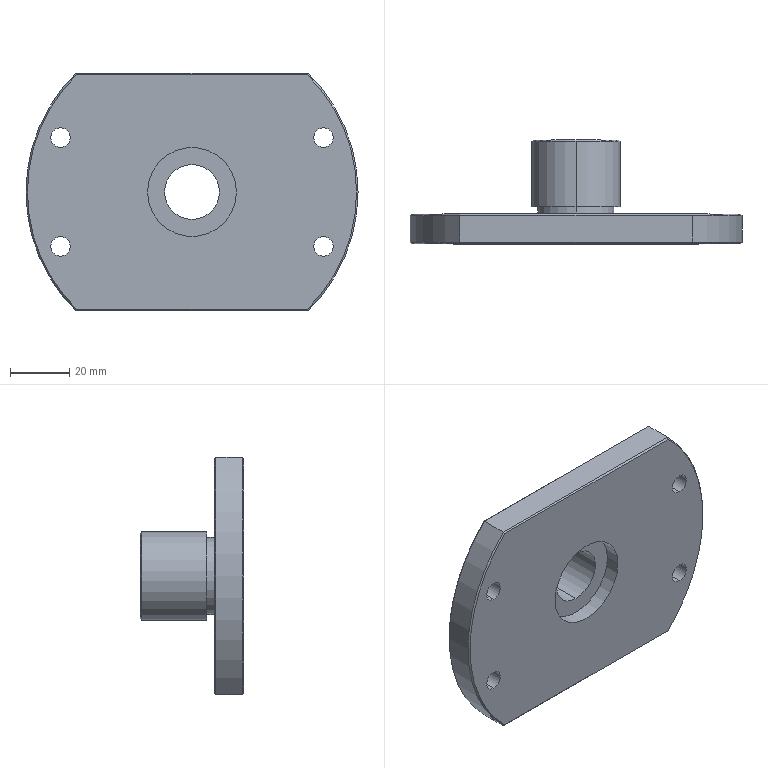Part | SolidWorks | features ICE 3, HoleWzd 2, Chamfer 1, Extrusion 1, RevCut 1 | 1 solid | 43 faces | box 112 x 35 x 80 mm | volume 84771 mm3 | cylinder 18 | cone 14 | plane 11 | commonest cylinder face diameters 6.6 x8 30 x4 18.5 x2 26 x2 112 x2
STEP:
#1=CARTESIAN_POINT('',(-15.,5.,0.));
#2=VERTEX_POINT('',#1);
#3=CARTESIAN_POINT('',(15.,5.,0.));
#4=VERTEX_POINT('',#3);
#5=CARTESIAN_POINT('',(0.,5.,0.));
#6=DIRECTION('',(0.,-1.,0.));
#7=DIRECTION('',(1.,0.,0.));
#8=AXIS2_PLACEMENT_3D('',#5,#6,#7);
#9=CIRCLE('',#8,15.);
#10=EDGE_CURVE('',#2,#4,#9,.T.);
#11=ORIENTED_EDGE('',*,*,#10,.F.);
#12=CARTESIAN_POINT('',(-15.,0.,0.));
#13=VERTEX_POINT('',#12);
#14=CARTESIAN_POINT('',(-15.,5.,0.));
#15=DIRECTION('',(0.,-1.,0.));
#16=VECTOR('',#15,1000.);
#17=LINE('',#14,#16);
#18=EDGE_CURVE('',#2,#13,#17,.T.);
#19=ORIENTED_EDGE('',*,*,#18,.T.);
#20=CARTESIAN_POINT('',(15.,0.,0.));
#21=VERTEX_POINT('',#20);
#22=CARTESIAN_POINT('',(0.,0.,0.));
#23=DIRECTION('',(0.,-1.,0.));
#24=DIRECTION('',(1.,0.,0.));
#25=AXIS2_PLACEMENT_3D('',#22,#23,#24);
#26=CIRCLE('',#25,15.);
#27=EDGE_CURVE('',#13,#21,#26,.T.);
#28=ORIENTED_EDGE('',*,*,#27,.T.);
#29=CARTESIAN_POINT('',(15.,5.,0.));
#30=DIRECTION('',(0.,-1.,0.));
#31=VECTOR('',#30,1000.);
#32=LINE('',#29,#31);
#33=EDGE_CURVE('',#4,#21,#32,.T.);
#34=ORIENTED_EDGE('',*,*,#33,.F.);
#35=EDGE_LOOP('',(#11,#19,#28,#34));
#36=FACE_OUTER_BOUND('',#35,.T.);
#37=CARTESIAN_POINT('',(0.,5.,0.));
#38=DIRECTION('',(0.,-1.,0.));
#39=DIRECTION('',(1.,0.,0.));
#40=AXIS2_PLACEMENT_3D('',#37,#38,#39);
#41=CYLINDRICAL_SURFACE('',#40,15.);
#42=ADVANCED_FACE('',(#36),#41,.F.);
#43=CARTESIAN_POINT('',(0.,35.,14.5));
#44=VERTEX_POINT('',#43);
#45=CARTESIAN_POINT('',(0.,35.,-14.5));
#46=VERTEX_POINT('',#45);
#47=CARTESIAN_POINT('',(0.,35.,0.));
#48=DIRECTION('',(0.,1.,0.));
#49=DIRECTION('',(0.,0.,1.));
#50=AXIS2_PLACEMENT_3D('',#47,#48,#49);
#51=CIRCLE('',#50,14.5);
#52=EDGE_CURVE('',#44,#46,#51,.T.);
#53=ORIENTED_EDGE('',*,*,#52,.F.);
#54=CARTESIAN_POINT('',(0.,34.5,15.));
#55=VERTEX_POINT('',#54);
#56=CARTESIAN_POINT('',(0.,35.,14.5));
#57=DIRECTION('',(0.,-0.7071,0.7071));
#58=VECTOR('',#57,1000.);
#59=LINE('',#56,#58);
#60=EDGE_CURVE('',#44,#55,#59,.T.);
#61=ORIENTED_EDGE('',*,*,#60,.T.);
#62=CARTESIAN_POINT('',(0.,34.5,-15.));
#63=VERTEX_POINT('',#62);
#64=CARTESIAN_POINT('',(0.,34.5,0.));
#65=DIRECTION('',(0.,-1.,0.));
#66=DIRECTION('',(0.,0.,1.));
#67=AXIS2_PLACEMENT_3D('',#64,#65,#66);
#68=CIRCLE('',#67,15.);
#69=EDGE_CURVE('',#63,#55,#68,.T.);
#70=ORIENTED_EDGE('',*,*,#69,.F.);
#71=CARTESIAN_POINT('',(0.,35.,-14.5));
#72=DIRECTION('',(0.,-0.7071,-0.7071));
#73=VECTOR('',#72,1000.);
#74=LINE('',#71,#73);
#75=EDGE_CURVE('',#46,#63,#74,.T.);
#76=ORIENTED_EDGE('',*,*,#75,.F.);
#77=EDGE_LOOP('',(#53,#61,#70,#76));
#78=FACE_OUTER_BOUND('',#77,.T.);
#79=CARTESIAN_POINT('',(0.,35.,0.));
#80=DIRECTION('',(0.,-1.,0.));
#81=DIRECTION('',(0.,0.,-1.));
#82=AXIS2_PLACEMENT_3D('',#79,#80,#81);
#83=CONICAL_SURFACE('',#82,14.5,0.7854);
#84=ADVANCED_FACE('',(#78),#83,.T.);
#85=CARTESIAN_POINT('',(0.,12.5,-13.));
#86=VERTEX_POINT('',#85);
#87=CARTESIAN_POINT('',(0.,12.5,13.));
#88=VERTEX_POINT('',#87);
#89=CARTESIAN_POINT('',(0.,12.5,0.));
#90=DIRECTION('',(0.,-1.,0.));
#91=DIRECTION('',(0.,0.,-1.));
#92=AXIS2_PLACEMENT_3D('',#89,#90,#91);
#93=CIRCLE('',#92,13.);
#94=EDGE_CURVE('',#86,#88,#93,.T.);
#95=ORIENTED_EDGE('',*,*,#94,.T.);
#96=CARTESIAN_POINT('',(0.,10.,13.));
#97=VERTEX_POINT('',#96);
#98=CARTESIAN_POINT('',(0.,-2.797,13.));
#99=DIRECTION('',(0.,-1.,0.));
#100=VECTOR('',#99,1000.);
#101=LINE('',#98,#100);
#102=EDGE_CURVE('',#88,#97,#101,.T.);
#103=ORIENTED_EDGE('',*,*,#102,.T.);
#104=CARTESIAN_POINT('',(0.,10.,-13.));
#105=VERTEX_POINT('',#104);
#106=CARTESIAN_POINT('',(0.,10.,0.));
#107=DIRECTION('',(0.,-1.,0.));
#108=DIRECTION('',(0.,0.,-1.));
#109=AXIS2_PLACEMENT_3D('',#106,#107,#108);
#110=CIRCLE('',#109,13.);
#111=EDGE_CURVE('',#105,#97,#110,.T.);
#112=ORIENTED_EDGE('',*,*,#111,.F.);
#113=CARTESIAN_POINT('',(0.,-2.797,-13.));
#114=DIRECTION('',(0.,-1.,0.));
#115=VECTOR('',#114,1000.);
#116=LINE('',#113,#115);
#117=EDGE_CURVE('',#86,#105,#116,.T.);
#118=ORIENTED_EDGE('',*,*,#117,.F.);
#119=EDGE_LOOP('',(#95,#103,#112,#118));
#120=FACE_OUTER_BOUND('',#119,.T.);
#121=CARTESIAN_POINT('',(0.,-2.797,0.));
#122=DIRECTION('',(0.,-1.,0.));
#123=DIRECTION('',(0.,0.,-1.));
#124=AXIS2_PLACEMENT_3D('',#121,#122,#123);
#125=CYLINDRICAL_SURFACE('',#124,13.);
#126=ADVANCED_FACE('',(#120),#125,.T.);
#127=CARTESIAN_POINT('',(44.346,6.58,15.069));
#128=VERTEX_POINT('',#127);
#129=CARTESIAN_POINT('',(44.346,6.58,21.669));
#130=VERTEX_POINT('',#129);
#131=CARTESIAN_POINT('',(44.346,6.58,18.369));
#132=DIRECTION('',(0.,1.,0.));
#133=DIRECTION('',(0.,0.,1.));
#134=AXIS2_PLACEMENT_3D('',#131,#132,#133);
#135=CIRCLE('',#134,3.3);
#136=EDGE_CURVE('',#128,#130,#135,.T.);
#137=ORIENTED_EDGE('',*,*,#136,.F.);
#138=CARTESIAN_POINT('',(44.346,10.,11.649));
#139=VERTEX_POINT('',#138);
#140=CARTESIAN_POINT('',(44.346,10.,11.649));
#141=DIRECTION('',(0.,0.7071,-0.7071));
#142=VECTOR('',#141,1000.);
#143=LINE('',#140,#142);
#144=EDGE_CURVE('',#128,#139,#143,.T.);
#145=ORIENTED_EDGE('',*,*,#144,.T.);
#146=CARTESIAN_POINT('',(44.346,10.,25.089));
#147=VERTEX_POINT('',#146);
#148=CARTESIAN_POINT('',(44.346,10.,18.369));
#149=DIRECTION('',(0.,1.,0.));
#150=DIRECTION('',(0.,0.,1.));
#151=AXIS2_PLACEMENT_3D('',#148,#149,#150);
#152=CIRCLE('',#151,6.72);
#153=EDGE_CURVE('',#139,#147,#152,.T.);
#154=ORIENTED_EDGE('',*,*,#153,.T.);
#155=CARTESIAN_POINT('',(44.346,10.,25.089));
#156=DIRECTION('',(0.,0.7071,0.7071));
#157=VECTOR('',#156,1000.);
#158=LINE('',#155,#157);
#159=EDGE_CURVE('',#130,#147,#158,.T.);
#160=ORIENTED_EDGE('',*,*,#159,.F.);
#161=EDGE_LOOP('',(#137,#145,#154,#160));
#162=FACE_OUTER_BOUND('',#161,.T.);
#163=CARTESIAN_POINT('',(44.346,10.,18.369));
#164=DIRECTION('',(0.,1.,0.));
#165=DIRECTION('',(0.,0.,1.));
#166=AXIS2_PLACEMENT_3D('',#163,#164,#165);
#167=CONICAL_SURFACE('',#166,6.72,0.7854);
#168=ADVANCED_FACE('',(#162),#167,.F.);
#169=CARTESIAN_POINT('',(44.346,0.,15.069));
#170=VERTEX_POINT('',#169);
#171=CARTESIAN_POINT('',(44.346,0.,21.669));
#172=VERTEX_POINT('',#171);
#173=CARTESIAN_POINT('',(44.346,0.,18.369));
#174=DIRECTION('',(0.,1.,0.));
#175=DIRECTION('',(0.,0.,1.));
#176=AXIS2_PLACEMENT_3D('',#173,#174,#175);
#177=CIRCLE('',#176,3.3);
#178=EDGE_CURVE('',#170,#172,#177,.T.);
#179=ORIENTED_EDGE('',*,*,#178,.F.);
#180=CARTESIAN_POINT('',(44.346,10.,15.069));
#181=DIRECTION('',(0.,1.,0.));
#182=VECTOR('',#181,1000.);
#183=LINE('',#180,#182);
#184=EDGE_CURVE('',#170,#128,#183,.T.);
#185=ORIENTED_EDGE('',*,*,#184,.T.);
#186=ORIENTED_EDGE('',*,*,#136,.T.);
#187=CARTESIAN_POINT('',(44.346,10.,21.669));
#188=DIRECTION('',(0.,1.,0.));
#189=VECTOR('',#188,1000.);
#190=LINE('',#187,#189);
#191=EDGE_CURVE('',#172,#130,#190,.T.);
#192=ORIENTED_EDGE('',*,*,#191,.F.);
#193=EDGE_LOOP('',(#179,#185,#186,#192));
#194=FACE_OUTER_BOUND('',#193,.T.);
#195=CARTESIAN_POINT('',(44.346,10.,18.369));
#196=DIRECTION('',(0.,1.,0.));
#197=DIRECTION('',(0.,0.,1.));
#198=AXIS2_PLACEMENT_3D('',#195,#196,#197);
#199=CYLINDRICAL_SURFACE('',#198,3.3);
#200=ADVANCED_FACE('',(#194),#199,.F.);
#201=CARTESIAN_POINT('',(-44.346,6.58,-21.669));
#202=VERTEX_POINT('',#201);
#203=CARTESIAN_POINT('',(-44.346,6.58,-15.069));
#204=VERTEX_POINT('',#203);
#205=CARTESIAN_POINT('',(-44.346,6.58,-18.369));
#206=DIRECTION('',(0.,1.,0.));
#207=DIRECTION('',(0.,0.,1.));
#208=AXIS2_PLACEMENT_3D('',#205,#206,#207);
#209=CIRCLE('',#208,3.3);
#210=EDGE_CURVE('',#202,#204,#209,.T.);
#211=ORIENTED_EDGE('',*,*,#210,.F.);
#212=CARTESIAN_POINT('',(-44.346,10.,-25.089));
#213=VERTEX_POINT('',#212);
#214=CARTESIAN_POINT('',(-44.346,10.,-25.089));
#215=DIRECTION('',(0.,0.7071,-0.7071));
#216=VECTOR('',#215,1000.);
#217=LINE('',#214,#216);
#218=EDGE_CURVE('',#202,#213,#217,.T.);
#219=ORIENTED_EDGE('',*,*,#218,.T.);
#220=CARTESIAN_POINT('',(-44.346,10.,-11.649));
#221=VERTEX_POINT('',#220);
#222=CARTESIAN_POINT('',(-44.346,10.,-18.369));
#223=DIRECTION('',(0.,1.,0.));
#224=DIRECTION('',(0.,0.,1.));
#225=AXIS2_PLACEMENT_3D('',#222,#223,#224);
#226=CIRCLE('',#225,6.72);
#227=EDGE_CURVE('',#213,#221,#226,.T.);
#228=ORIENTED_EDGE('',*,*,#227,.T.);
#229=CARTESIAN_POINT('',(-44.346,10.,-11.649));
#230=DIRECTION('',(0.,0.7071,0.7071));
#231=VECTOR('',#230,1000.);
#232=LINE('',#229,#231);
#233=EDGE_CURVE('',#204,#221,#232,.T.);
#234=ORIENTED_EDGE('',*,*,#233,.F.);
#235=EDGE_LOOP('',(#211,#219,#228,#234));
#236=FACE_OUTER_BOUND('',#235,.T.);
#237=CARTESIAN_POINT('',(-44.346,10.,-18.369));
#238=DIRECTION('',(0.,1.,0.));
#239=DIRECTION('',(0.,0.,1.));
#240=AXIS2_PLACEMENT_3D('',#237,#238,#239);
#241=CONICAL_SURFACE('',#240,6.72,0.7854);
#242=ADVANCED_FACE('',(#236),#241,.F.);
#243=CARTESIAN_POINT('',(-44.346,0.,-21.669));
#244=VERTEX_POINT('',#243);
#245=CARTESIAN_POINT('',(-44.346,0.,-15.069));
#246=VERTEX_POINT('',#245);
#247=CARTESIAN_POINT('',(-44.346,0.,-18.369));
#248=DIRECTION('',(0.,1.,0.));
#249=DIRECTION('',(0.,0.,1.));
#250=AXIS2_PLACEMENT_3D('',#247,#248,#249);
#251=CIRCLE('',#250,3.3);
#252=EDGE_CURVE('',#244,#246,#251,.T.);
#253=ORIENTED_EDGE('',*,*,#252,.F.);
#254=CARTESIAN_POINT('',(-44.346,10.,-21.669));
#255=DIRECTION('',(0.,1.,0.));
#256=VECTOR('',#255,1000.);
#257=LINE('',#254,#256);
#258=EDGE_CURVE('',#244,#202,#257,.T.);
#259=ORIENTED_EDGE('',*,*,#258,.T.);
#260=ORIENTED_EDGE('',*,*,#210,.T.);
#261=CARTESIAN_POINT('',(-44.346,10.,-15.069));
#262=DIRECTION('',(0.,1.,0.));
#263=VECTOR('',#262,1000.);
#264=LINE('',#261,#263);
#265=EDGE_CURVE('',#246,#204,#264,.T.);
#266=ORIENTED_EDGE('',*,*,#265,.F.);
#267=EDGE_LOOP('',(#253,#259,#260,#266));
#268=FACE_OUTER_BOUND('',#267,.T.);
#269=CARTESIAN_POINT('',(-44.346,10.,-18.369));
#270=DIRECTION('',(0.,1.,0.));
#271=DIRECTION('',(0.,0.,1.));
#272=AXIS2_PLACEMENT_3D('',#269,#270,#271);
#273=CYLINDRICAL_SURFACE('',#272,3.3);
#274=ADVANCED_FACE('',(#268),#273,.F.);
#275=CARTESIAN_POINT('',(-44.346,6.58,15.069));
#276=VERTEX_POINT('',#275);
#277=CARTESIAN_POINT('',(-44.346,6.58,21.669));
#278=VERTEX_POINT('',#277);
#279=CARTESIAN_POINT('',(-44.346,6.58,18.369));
#280=DIRECTION('',(0.,1.,0.));
#281=DIRECTION('',(0.,0.,1.));
#282=AXIS2_PLACEMENT_3D('',#279,#280,#281);
#283=CIRCLE('',#282,3.3);
#284=EDGE_CURVE('',#276,#278,#283,.T.);
#285=ORIENTED_EDGE('',*,*,#284,.F.);
#286=CARTESIAN_POINT('',(-44.346,10.,11.649));
#287=VERTEX_POINT('',#286);
#288=CARTESIAN_POINT('',(-44.346,10.,11.649));
#289=DIRECTION('',(0.,0.7071,-0.7071));
#290=VECTOR('',#289,1000.);
#291=LINE('',#288,#290);
#292=EDGE_CURVE('',#276,#287,#291,.T.);
#293=ORIENTED_EDGE('',*,*,#292,.T.);
#294=CARTESIAN_POINT('',(-44.346,10.,25.089));
#295=VERTEX_POINT('',#294);
#296=CARTESIAN_POINT('',(-44.346,10.,18.369));
#297=DIRECTION('',(0.,1.,0.));
#298=DIRECTION('',(0.,0.,1.));
#299=AXIS2_PLACEMENT_3D('',#296,#297,#298);
#300=CIRCLE('',#299,6.72);
#301=EDGE_CURVE('',#287,#295,#300,.T.);
#302=ORIENTED_EDGE('',*,*,#301,.T.);
#303=CARTESIAN_POINT('',(-44.346,10.,25.089));
#304=DIRECTION('',(0.,0.7071,0.7071));
#305=VECTOR('',#304,1000.);
#306=LINE('',#303,#305);
#307=EDGE_CURVE('',#278,#295,#306,.T.);
#308=ORIENTED_EDGE('',*,*,#307,.F.);
#309=EDGE_LOOP('',(#285,#293,#302,#308));
#310=FACE_OUTER_BOUND('',#309,.T.);
#311=CARTESIAN_POINT('',(-44.346,10.,18.369));
#312=DIRECTION('',(0.,1.,0.));
#313=DIRECTION('',(0.,0.,1.));
#314=AXIS2_PLACEMENT_3D('',#311,#312,#313);
#315=CONICAL_SURFACE('',#314,6.72,0.7854);
#316=ADVANCED_FACE('',(#310),#315,.F.);
#317=CARTESIAN_POINT('',(-44.346,0.,15.069));
#318=VERTEX_POINT('',#317);
#319=CARTESIAN_POINT('',(-44.346,0.,21.669));
#320=VERTEX_POINT('',#319);
#321=CARTESIAN_POINT('',(-44.346,0.,18.369));
#322=DIRECTION('',(0.,1.,0.));
#323=DIRECTION('',(0.,0.,1.));
#324=AXIS2_PLACEMENT_3D('',#321,#322,#323);
#325=CIRCLE('',#324,3.3);
#326=EDGE_CURVE('',#318,#320,#325,.T.);
#327=ORIENTED_EDGE('',*,*,#326,.F.);
#328=CARTESIAN_POINT('',(-44.346,10.,15.069));
#329=DIRECTION('',(0.,1.,0.));
#330=VECTOR('',#329,1000.);
#331=LINE('',#328,#330);
#332=EDGE_CURVE('',#318,#276,#331,.T.);
#333=ORIENTED_EDGE('',*,*,#332,.T.);
#334=ORIENTED_EDGE('',*,*,#284,.T.);
#335=CARTESIAN_POINT('',(-44.346,10.,21.669));
#336=DIRECTION('',(0.,1.,0.));
#337=VECTOR('',#336,1000.);
#338=LINE('',#335,#337);
#339=EDGE_CURVE('',#320,#278,#338,.T.);
#340=ORIENTED_EDGE('',*,*,#339,.F.);
#341=EDGE_LOOP('',(#327,#333,#334,#340));
#342=FACE_OUTER_BOUND('',#341,.T.);
#343=CARTESIAN_POINT('',(-44.346,10.,18.369));
#344=DIRECTION('',(0.,1.,0.));
#345=DIRECTION('',(0.,0.,1.));
#346=AXIS2_PLACEMENT_3D('',#343,#344,#345);
#347=CYLINDRICAL_SURFACE('',#346,3.3);
#348=ADVANCED_FACE('',(#342),#347,.F.);
#349=CARTESIAN_POINT('',(44.346,6.58,-21.669));
#350=VERTEX_POINT('',#349);
#351=CARTESIAN_POINT('',(44.346,6.58,-15.069));
#352=VERTEX_POINT('',#351);
#353=CARTESIAN_POINT('',(44.346,6.58,-18.369));
#354=DIRECTION('',(0.,1.,0.));
#355=DIRECTION('',(0.,0.,1.));
#356=AXIS2_PLACEMENT_3D('',#353,#354,#355);
#357=CIRCLE('',#356,3.3);
#358=EDGE_CURVE('',#350,#352,#357,.T.);
#359=ORIENTED_EDGE('',*,*,#358,.F.);
#360=CARTESIAN_POINT('',(44.346,10.,-25.089));
#361=VERTEX_POINT('',#360);
#362=CARTESIAN_POINT('',(44.346,10.,-25.089));
#363=DIRECTION('',(0.,0.7071,-0.7071));
#364=VECTOR('',#363,1000.);
#365=LINE('',#362,#364);
#366=EDGE_CURVE('',#350,#361,#365,.T.);
#367=ORIENTED_EDGE('',*,*,#366,.T.);
#368=CARTESIAN_POINT('',(44.346,10.,-11.649));
#369=VERTEX_POINT('',#368);
#370=CARTESIAN_POINT('',(44.346,10.,-18.369));
#371=DIRECTION('',(0.,1.,0.));
#372=DIRECTION('',(0.,0.,1.));
#373=AXIS2_PLACEMENT_3D('',#370,#371,#372);
#374=CIRCLE('',#373,6.72);
#375=EDGE_CURVE('',#361,#369,#374,.T.);
#376=ORIENTED_EDGE('',*,*,#375,.T.);
#377=CARTESIAN_POINT('',(44.346,10.,-11.649));
#378=DIRECTION('',(0.,0.7071,0.7071));
#379=VECTOR('',#378,1000.);
#380=LINE('',#377,#379);
#381=EDGE_CURVE('',#352,#369,#380,.T.);
#382=ORIENTED_EDGE('',*,*,#381,.F.);
#383=EDGE_LOOP('',(#359,#367,#376,#382));
#384=FACE_OUTER_BOUND('',#383,.T.);
#385=CARTESIAN_POINT('',(44.346,10.,-18.369));
#386=DIRECTION('',(0.,1.,0.));
#387=DIRECTION('',(0.,0.,1.));
#388=AXIS2_PLACEMENT_3D('',#385,#386,#387);
#389=CONICAL_SURFACE('',#388,6.72,0.7854);
#390=ADVANCED_FACE('',(#384),#389,.F.);
#391=CARTESIAN_POINT('',(44.346,0.,-21.669));
#392=VERTEX_POINT('',#391);
#393=CARTESIAN_POINT('',(44.346,0.,-15.069));
#394=VERTEX_POINT('',#393);
#395=CARTESIAN_POINT('',(44.346,0.,-18.369));
#396=DIRECTION('',(0.,1.,0.));
#397=DIRECTION('',(0.,0.,1.));
#398=AXIS2_PLACEMENT_3D('',#395,#396,#397);
#399=CIRCLE('',#398,3.3);
#400=EDGE_CURVE('',#392,#394,#399,.T.);
#401=ORIENTED_EDGE('',*,*,#400,.F.);
#402=CARTESIAN_POINT('',(44.346,10.,-21.669));
#403=DIRECTION('',(0.,1.,0.));
#404=VECTOR('',#403,1000.);
#405=LINE('',#402,#404);
#406=EDGE_CURVE('',#392,#350,#405,.T.);
#407=ORIENTED_EDGE('',*,*,#406,.T.);
#408=ORIENTED_EDGE('',*,*,#358,.T.);
#409=CARTESIAN_POINT('',(44.346,10.,-15.069));
#410=DIRECTION('',(0.,1.,0.));
#411=VECTOR('',#410,1000.);
#412=LINE('',#409,#411);
#413=EDGE_CURVE('',#394,#352,#412,.T.);
#414=ORIENTED_EDGE('',*,*,#413,.F.);
#415=EDGE_LOOP('',(#401,#407,#408,#414));
#416=FACE_OUTER_BOUND('',#415,.T.);
#417=CARTESIAN_POINT('',(44.346,10.,-18.369));
#418=DIRECTION('',(0.,1.,0.));
#419=DIRECTION('',(0.,0.,1.));
#420=AXIS2_PLACEMENT_3D('',#417,#418,#419);
#421=CYLINDRICAL_SURFACE('',#420,3.3);
#422=ADVANCED_FACE('',(#416),#421,.F.);
#423=ORIENTED_EDGE('',*,*,#69,.T.);
#424=CARTESIAN_POINT('',(0.,12.5,15.));
#425=VERTEX_POINT('',#424);
#426=CARTESIAN_POINT('',(0.,35.,15.));
#427=DIRECTION('',(0.,-1.,0.));
#428=VECTOR('',#427,1000.);
#429=LINE('',#426,#428);
#430=EDGE_CURVE('',#55,#425,#429,.T.);
#431=ORIENTED_EDGE('',*,*,#430,.T.);
#432=CARTESIAN_POINT('',(0.,12.5,-15.));
#433=VERTEX_POINT('',#432);
#434=CARTESIAN_POINT('',(0.,12.5,0.));
#435=DIRECTION('',(0.,-1.,0.));
#436=DIRECTION('',(0.,0.,-1.));
#437=AXIS2_PLACEMENT_3D('',#434,#435,#436);
#438=CIRCLE('',#437,15.);
#439=EDGE_CURVE('',#433,#425,#438,.T.);
#440=ORIENTED_EDGE('',*,*,#439,.F.);
#441=CARTESIAN_POINT('',(0.,35.,-15.));
#442=DIRECTION('',(0.,-1.,0.));
#443=VECTOR('',#442,1000.);
#444=LINE('',#441,#443);
#445=EDGE_CURVE('',#63,#433,#444,.T.);
#446=ORIENTED_EDGE('',*,*,#445,.F.);
#447=EDGE_LOOP('',(#423,#431,#440,#446));
#448=FACE_OUTER_BOUND('',#447,.T.);
#449=CARTESIAN_POINT('',(0.,35.,0.));
#450=DIRECTION('',(0.,-1.,0.));
#451=DIRECTION('',(0.,0.,-1.));
#452=AXIS2_PLACEMENT_3D('',#449,#450,#451);
#453=CYLINDRICAL_SURFACE('',#452,15.);
#454=ADVANCED_FACE('',(#448),#453,.T.);
#455=CARTESIAN_POINT('',(0.,5.,-9.25));
#456=VERTEX_POINT('',#455);
#457=CARTESIAN_POINT('',(0.,5.,9.25));
#458=VERTEX_POINT('',#457);
#459=CARTESIAN_POINT('',(0.,5.,0.));
#460=DIRECTION('',(0.,1.,0.));
#461=DIRECTION('',(1.,0.,0.));
#462=AXIS2_PLACEMENT_3D('',#459,#460,#461);
#463=CIRCLE('',#462,9.25);
#464=EDGE_CURVE('',#456,#458,#463,.T.);
#465=ORIENTED_EDGE('',*,*,#464,.F.);
#466=CARTESIAN_POINT('',(0.,35.,-9.25));
#467=VERTEX_POINT('',#466);
#468=CARTESIAN_POINT('',(0.,35.,-9.25));
#469=DIRECTION('',(0.,1.,0.));
#470=VECTOR('',#469,1000.);
#471=LINE('',#468,#470);
#472=EDGE_CURVE('',#456,#467,#471,.T.);
#473=ORIENTED_EDGE('',*,*,#472,.T.);
#474=CARTESIAN_POINT('',(0.,35.,9.25));
#475=VERTEX_POINT('',#474);
#476=CARTESIAN_POINT('',(0.,35.,0.));
#477=DIRECTION('',(0.,1.,0.));
#478=DIRECTION('',(0.,0.,1.));
#479=AXIS2_PLACEMENT_3D('',#476,#477,#478);
#480=CIRCLE('',#479,9.25);
#481=EDGE_CURVE('',#467,#475,#480,.T.);
#482=ORIENTED_EDGE('',*,*,#481,.T.);
#483=CARTESIAN_POINT('',(0.,35.,9.25));
#484=DIRECTION('',(0.,1.,0.));
#485=VECTOR('',#484,1000.);
#486=LINE('',#483,#485);
#487=EDGE_CURVE('',#458,#475,#486,.T.);
#488=ORIENTED_EDGE('',*,*,#487,.F.);
#489=EDGE_LOOP('',(#465,#473,#482,#488));
#490=FACE_OUTER_BOUND('',#489,.T.);
#491=CARTESIAN_POINT('',(0.,35.,0.));
#492=DIRECTION('',(0.,1.,0.));
#493=DIRECTION('',(0.,0.,1.));
#494=AXIS2_PLACEMENT_3D('',#491,#492,#493);
#495=CYLINDRICAL_SURFACE('',#494,9.25);
#496=ADVANCED_FACE('',(#490),#495,.F.);
#497=ORIENTED_EDGE('',*,*,#472,.F.);
#498=CARTESIAN_POINT('',(0.,5.,0.));
#499=DIRECTION('',(0.,1.,0.));
#500=DIRECTION('',(1.,0.,0.));
#501=AXIS2_PLACEMENT_3D('',#498,#499,#500);
#502=CIRCLE('',#501,9.25);
#503=EDGE_CURVE('',#458,#456,#502,.T.);
#504=ORIENTED_EDGE('',*,*,#503,.F.);
#505=ORIENTED_EDGE('',*,*,#487,.T.);
#506=CARTESIAN_POINT('',(0.,35.,0.));
#507=DIRECTION('',(0.,1.,0.));
#508=DIRECTION('',(0.,0.,1.));
#509=AXIS2_PLACEMENT_3D('',#506,#507,#508);
#510=CIRCLE('',#509,9.25);
#511=EDGE_CURVE('',#475,#467,#510,.T.);
#512=ORIENTED_EDGE('',*,*,#511,.T.);
#513=EDGE_LOOP('',(#497,#504,#505,#512));
#514=FACE_OUTER_BOUND('',#513,.T.);
#515=CARTESIAN_POINT('',(0.,35.,0.));
#516=DIRECTION('',(0.,1.,0.));
#517=DIRECTION('',(0.,0.,1.));
#518=AXIS2_PLACEMENT_3D('',#515,#516,#517);
#519=CYLINDRICAL_SURFACE('',#518,9.25);
#520=ADVANCED_FACE('',(#514),#519,.F.);
#521=ORIENTED_EDGE('',*,*,#430,.F.);
#522=CARTESIAN_POINT('',(0.,34.5,0.));
#523=DIRECTION('',(0.,-1.,0.));
#524=DIRECTION('',(0.,0.,1.));
#525=AXIS2_PLACEMENT_3D('',#522,#523,#524);
#526=CIRCLE('',#525,15.);
#527=EDGE_CURVE('',#55,#63,#526,.T.);
#528=ORIENTED_EDGE('',*,*,#527,.T.);
#529=ORIENTED_EDGE('',*,*,#445,.T.);
#530=CARTESIAN_POINT('',(0.,12.5,0.));
#531=DIRECTION('',(0.,-1.,0.));
#532=DIRECTION('',(0.,0.,-1.));
#533=AXIS2_PLACEMENT_3D('',#530,#531,#532);
#534=CIRCLE('',#533,15.);
#535=EDGE_CURVE('',#425,#433,#534,.T.);
#536=ORIENTED_EDGE('',*,*,#535,.F.);
#537=EDGE_LOOP('',(#521,#528,#529,#536));
#538=FACE_OUTER_BOUND('',#537,.T.);
#539=CARTESIAN_POINT('',(0.,35.,0.));
#540=DIRECTION('',(0.,-1.,0.));
#541=DIRECTION('',(0.,0.,-1.));
#542=AXIS2_PLACEMENT_3D('',#539,#540,#541);
#543=CYLINDRICAL_SURFACE('',#542,15.);
#544=ADVANCED_FACE('',(#538),#543,.T.);
#545=CARTESIAN_POINT('',(-38.987,10.,39.5));
#546=VERTEX_POINT('',#545);
#547=CARTESIAN_POINT('',(38.987,10.,39.5));
#548=VERTEX_POINT('',#547);
#549=CARTESIAN_POINT('',(0.,10.,39.5));
#550=DIRECTION('',(1.,0.,0.));
#551=VECTOR('',#550,1000.);
#552=LINE('',#549,#551);
#553=EDGE_CURVE('',#546,#548,#552,.T.);
#554=ORIENTED_EDGE('',*,*,#553,.T.);
#555=CARTESIAN_POINT('',(38.987,10.,-39.5));
#556=VERTEX_POINT('',#555);
#557=CARTESIAN_POINT('',(0.,10.,0.));
#558=DIRECTION('',(0.,1.,0.));
#559=DIRECTION('',(0.,0.,1.));
#560=AXIS2_PLACEMENT_3D('',#557,#558,#559);
#561=CIRCLE('',#560,55.5);
#562=EDGE_CURVE('',#548,#556,#561,.T.);
#563=ORIENTED_EDGE('',*,*,#562,.T.);
#564=CARTESIAN_POINT('',(-38.987,10.,-39.5));
#565=VERTEX_POINT('',#564);
#566=CARTESIAN_POINT('',(0.,10.,-39.5));
#567=DIRECTION('',(-1.,0.,0.));
#568=VECTOR('',#567,1000.);
#569=LINE('',#566,#568);
#570=EDGE_CURVE('',#556,#565,#569,.T.);
#571=ORIENTED_EDGE('',*,*,#570,.T.);
#572=CARTESIAN_POINT('',(0.,10.,0.));
#573=DIRECTION('',(0.,1.,0.));
#574=DIRECTION('',(0.,0.,1.));
#575=AXIS2_PLACEMENT_3D('',#572,#573,#574);
#576=CIRCLE('',#575,55.5);
#577=EDGE_CURVE('',#565,#546,#576,.T.);
#578=ORIENTED_EDGE('',*,*,#577,.T.);
#579=EDGE_LOOP('',(#554,#563,#571,#578));
#580=FACE_OUTER_BOUND('',#579,.T.);
#581=CARTESIAN_POINT('',(44.346,10.,18.369));
#582=DIRECTION('',(0.,1.,0.));
#583=DIRECTION('',(0.,0.,1.));
#584=AXIS2_PLACEMENT_3D('',#581,#582,#583);
#585=CIRCLE('',#584,6.72);
#586=EDGE_CURVE('',#147,#139,#585,.T.);
#587=ORIENTED_EDGE('',*,*,#586,.F.);
#588=ORIENTED_EDGE('',*,*,#153,.F.);
#589=EDGE_LOOP('',(#587,#588));
#590=FACE_BOUND('',#589,.T.);
#591=CARTESIAN_POINT('',(-44.346,10.,-18.369));
#592=DIRECTION('',(0.,1.,0.));
#593=DIRECTION('',(0.,0.,1.));
#594=AXIS2_PLACEMENT_3D('',#591,#592,#593);
#595=CIRCLE('',#594,6.72);
#596=EDGE_CURVE('',#221,#213,#595,.T.);
#597=ORIENTED_EDGE('',*,*,#596,.F.);
#598=ORIENTED_EDGE('',*,*,#227,.F.);
#599=EDGE_LOOP('',(#597,#598));
#600=FACE_BOUND('',#599,.T.);
#601=CARTESIAN_POINT('',(-44.346,10.,18.369));
#602=DIRECTION('',(0.,1.,0.));
#603=DIRECTION('',(0.,0.,1.));
#604=AXIS2_PLACEMENT_3D('',#601,#602,#603);
#605=CIRCLE('',#604,6.72);
#606=EDGE_CURVE('',#295,#287,#605,.T.);
#607=ORIENTED_EDGE('',*,*,#606,.F.);
#608=ORIENTED_EDGE('',*,*,#301,.F.);
#609=EDGE_LOOP('',(#607,#608));
#610=FACE_BOUND('',#609,.T.);
#611=CARTESIAN_POINT('',(44.346,10.,-18.369));
#612=DIRECTION('',(0.,1.,0.));
#613=DIRECTION('',(0.,0.,1.));
#614=AXIS2_PLACEMENT_3D('',#611,#612,#613);
#615=CIRCLE('',#614,6.72);
#616=EDGE_CURVE('',#369,#361,#615,.T.);
#617=ORIENTED_EDGE('',*,*,#616,.F.);
#618=ORIENTED_EDGE('',*,*,#375,.F.);
#619=EDGE_LOOP('',(#617,#618));
#620=FACE_BOUND('',#619,.T.);
#621=ORIENTED_EDGE('',*,*,#111,.T.);
#622=CARTESIAN_POINT('',(0.,10.,0.));
#623=DIRECTION('',(0.,-1.,0.));
#624=DIRECTION('',(0.,0.,-1.));
#625=AXIS2_PLACEMENT_3D('',#622,#623,#624);
#626=CIRCLE('',#625,13.);
#627=EDGE_CURVE('',#97,#105,#626,.T.);
#628=ORIENTED_EDGE('',*,*,#627,.T.);
#629=EDGE_LOOP('',(#621,#628));
#630=FACE_BOUND('',#629,.T.);
#631=CARTESIAN_POINT('',(0.,10.,0.));
#632=DIRECTION('',(0.,1.,0.));
#633=DIRECTION('',(0.,0.,1.));
#634=AXIS2_PLACEMENT_3D('',#631,#632,#633);
#635=PLANE('',#634);
#636=ADVANCED_FACE('',(#580,#590,#600,#610,#620,#630),#635,.T.);
#637=CARTESIAN_POINT('',(-39.192,9.5,40.));
#638=VERTEX_POINT('',#637);
#639=CARTESIAN_POINT('',(-39.192,0.5,40.));
#640=VERTEX_POINT('',#639);
#641=CARTESIAN_POINT('',(-39.192,10.,40.));
#642=DIRECTION('',(0.,-1.,0.));
#643=VECTOR('',#642,1000.);
#644=LINE('',#641,#643);
#645=EDGE_CURVE('',#638,#640,#644,.T.);
#646=ORIENTED_EDGE('',*,*,#645,.F.);
#647=CARTESIAN_POINT('',(-39.192,9.5,-40.));
#648=VERTEX_POINT('',#647);
#649=CARTESIAN_POINT('',(0.,9.5,0.));
#650=DIRECTION('',(0.,-1.,0.));
#651=DIRECTION('',(0.,0.,1.));
#652=AXIS2_PLACEMENT_3D('',#649,#650,#651);
#653=CIRCLE('',#652,56.);
#654=EDGE_CURVE('',#638,#648,#653,.T.);
#655=ORIENTED_EDGE('',*,*,#654,.T.);
#656=CARTESIAN_POINT('',(-39.192,0.5,-40.));
#657=VERTEX_POINT('',#656);
#658=CARTESIAN_POINT('',(-39.192,10.,-40.));
#659=DIRECTION('',(0.,1.,0.));
#660=VECTOR('',#659,1000.);
#661=LINE('',#658,#660);
#662=EDGE_CURVE('',#657,#648,#661,.T.);
#663=ORIENTED_EDGE('',*,*,#662,.F.);
#664=CARTESIAN_POINT('',(0.,0.5,0.));
#665=DIRECTION('',(0.,1.,0.));
#666=DIRECTION('',(0.,0.,1.));
#667=AXIS2_PLACEMENT_3D('',#664,#665,#666);
#668=CIRCLE('',#667,56.);
#669=EDGE_CURVE('',#657,#640,#668,.T.);
#670=ORIENTED_EDGE('',*,*,#669,.T.);
#671=EDGE_LOOP('',(#646,#655,#663,#670));
#672=FACE_OUTER_BOUND('',#671,.T.);
#673=CARTESIAN_POINT('',(0.,10.,0.));
#674=DIRECTION('',(0.,-1.,0.));
#675=DIRECTION('',(0.,0.,-1.));
#676=AXIS2_PLACEMENT_3D('',#673,#674,#675);
#677=CYLINDRICAL_SURFACE('',#676,56.);
#678=ADVANCED_FACE('',(#672),#677,.T.);
#679=CARTESIAN_POINT('',(39.192,9.5,-40.));
#680=VERTEX_POINT('',#679);
#681=CARTESIAN_POINT('',(39.192,0.5,-40.));
#682=VERTEX_POINT('',#681);
#683=CARTESIAN_POINT('',(39.192,10.,-40.));
#684=DIRECTION('',(0.,-1.,0.));
#685=VECTOR('',#684,1000.);
#686=LINE('',#683,#685);
#687=EDGE_CURVE('',#680,#682,#686,.T.);
#688=ORIENTED_EDGE('',*,*,#687,.F.);
#689=CARTESIAN_POINT('',(39.192,9.5,40.));
#690=VERTEX_POINT('',#689);
#691=CARTESIAN_POINT('',(0.,9.5,0.));
#692=DIRECTION('',(0.,-1.,0.));
#693=DIRECTION('',(0.,0.,1.));
#694=AXIS2_PLACEMENT_3D('',#691,#692,#693);
#695=CIRCLE('',#694,56.);
#696=EDGE_CURVE('',#680,#690,#695,.T.);
#697=ORIENTED_EDGE('',*,*,#696,.T.);
#698=CARTESIAN_POINT('',(39.192,0.5,40.));
#699=VERTEX_POINT('',#698);
#700=CARTESIAN_POINT('',(39.192,10.,40.));
#701=DIRECTION('',(0.,1.,0.));
#702=VECTOR('',#701,1000.);
#703=LINE('',#700,#702);
#704=EDGE_CURVE('',#699,#690,#703,.T.);
#705=ORIENTED_EDGE('',*,*,#704,.F.);
#706=CARTESIAN_POINT('',(0.,0.5,0.));
#707=DIRECTION('',(0.,1.,0.));
#708=DIRECTION('',(0.,0.,1.));
#709=AXIS2_PLACEMENT_3D('',#706,#707,#708);
#710=CIRCLE('',#709,56.);
#711=EDGE_CURVE('',#699,#682,#710,.T.);
#712=ORIENTED_EDGE('',*,*,#711,.T.);
#713=EDGE_LOOP('',(#688,#697,#705,#712));
#714=FACE_OUTER_BOUND('',#713,.T.);
#715=CARTESIAN_POINT('',(0.,10.,0.));
#716=DIRECTION('',(0.,-1.,0.));
#717=DIRECTION('',(0.,0.,-1.));
#718=AXIS2_PLACEMENT_3D('',#715,#716,#717);
#719=CYLINDRICAL_SURFACE('',#718,56.);
#720=ADVANCED_FACE('',(#714),#719,.T.);
#721=CARTESIAN_POINT('',(0.,0.,0.));
#722=DIRECTION('',(0.,-1.,0.));
#723=DIRECTION('',(1.,0.,0.));
#724=AXIS2_PLACEMENT_3D('',#721,#722,#723);
#725=CIRCLE('',#724,15.);
#726=EDGE_CURVE('',#21,#13,#725,.T.);
#727=ORIENTED_EDGE('',*,*,#726,.F.);
#728=ORIENTED_EDGE('',*,*,#27,.F.);
#729=EDGE_LOOP('',(#727,#728));
#730=FACE_BOUND('',#729,.T.);
#731=CARTESIAN_POINT('',(38.987,0.,39.5));
#732=VERTEX_POINT('',#731);
#733=CARTESIAN_POINT('',(-38.987,0.,39.5));
#734=VERTEX_POINT('',#733);
#735=CARTESIAN_POINT('',(-39.192,0.,39.5));
#736=DIRECTION('',(-1.,0.,0.));
#737=VECTOR('',#736,1000.);
#738=LINE('',#735,#737);
#739=EDGE_CURVE('',#732,#734,#738,.T.);
#740=ORIENTED_EDGE('',*,*,#739,.T.);
#741=CARTESIAN_POINT('',(-38.987,0.,-39.5));
#742=VERTEX_POINT('',#741);
#743=CARTESIAN_POINT('',(0.,0.,0.));
#744=DIRECTION('',(0.,-1.,0.));
#745=DIRECTION('',(0.,0.,1.));
#746=AXIS2_PLACEMENT_3D('',#743,#744,#745);
#747=CIRCLE('',#746,55.5);
#748=EDGE_CURVE('',#734,#742,#747,.T.);
#749=ORIENTED_EDGE('',*,*,#748,.T.);
#750=CARTESIAN_POINT('',(38.987,0.,-39.5));
#751=VERTEX_POINT('',#750);
#752=CARTESIAN_POINT('',(39.192,0.,-39.5));
#753=DIRECTION('',(1.,0.,0.));
#754=VECTOR('',#753,1000.);
#755=LINE('',#752,#754);
#756=EDGE_CURVE('',#742,#751,#755,.T.);
#757=ORIENTED_EDGE('',*,*,#756,.T.);
#758=CARTESIAN_POINT('',(0.,0.,0.));
#759=DIRECTION('',(0.,-1.,0.));
#760=DIRECTION('',(0.,0.,1.));
#761=AXIS2_PLACEMENT_3D('',#758,#759,#760);
#762=CIRCLE('',#761,55.5);
#763=EDGE_CURVE('',#751,#732,#762,.T.);
#764=ORIENTED_EDGE('',*,*,#763,.T.);
#765=EDGE_LOOP('',(#740,#749,#757,#764));
#766=FACE_OUTER_BOUND('',#765,.T.);
#767=CARTESIAN_POINT('',(44.346,0.,18.369));
#768=DIRECTION('',(0.,1.,0.));
#769=DIRECTION('',(0.,0.,1.));
#770=AXIS2_PLACEMENT_3D('',#767,#768,#769);
#771=CIRCLE('',#770,3.3);
#772=EDGE_CURVE('',#172,#170,#771,.T.);
#773=ORIENTED_EDGE('',*,*,#772,.T.);
#774=ORIENTED_EDGE('',*,*,#178,.T.);
#775=EDGE_LOOP('',(#773,#774));
#776=FACE_BOUND('',#775,.T.);
#777=CARTESIAN_POINT('',(-44.346,0.,-18.369));
#778=DIRECTION('',(0.,1.,0.));
#779=DIRECTION('',(0.,0.,1.));
#780=AXIS2_PLACEMENT_3D('',#777,#778,#779);
#781=CIRCLE('',#780,3.3);
#782=EDGE_CURVE('',#246,#244,#781,.T.);
#783=ORIENTED_EDGE('',*,*,#782,.T.);
#784=ORIENTED_EDGE('',*,*,#252,.T.);
#785=EDGE_LOOP('',(#783,#784));
#786=FACE_BOUND('',#785,.T.);
#787=CARTESIAN_POINT('',(-44.346,0.,18.369));
#788=DIRECTION('',(0.,1.,0.));
#789=DIRECTION('',(0.,0.,1.));
#790=AXIS2_PLACEMENT_3D('',#787,#788,#789);
#791=CIRCLE('',#790,3.3);
#792=EDGE_CURVE('',#320,#318,#791,.T.);
#793=ORIENTED_EDGE('',*,*,#792,.T.);
#794=ORIENTED_EDGE('',*,*,#326,.T.);
#795=EDGE_LOOP('',(#793,#794));
#796=FACE_BOUND('',#795,.T.);
#797=CARTESIAN_POINT('',(44.346,0.,-18.369));
#798=DIRECTION('',(0.,1.,0.));
#799=DIRECTION('',(0.,0.,1.));
#800=AXIS2_PLACEMENT_3D('',#797,#798,#799);
#801=CIRCLE('',#800,3.3);
#802=EDGE_CURVE('',#394,#392,#801,.T.);
#803=ORIENTED_EDGE('',*,*,#802,.T.);
#804=ORIENTED_EDGE('',*,*,#400,.T.);
#805=EDGE_LOOP('',(#803,#804));
#806=FACE_BOUND('',#805,.T.);
#807=CARTESIAN_POINT('',(0.,0.,0.));
#808=DIRECTION('',(0.,1.,0.));
#809=DIRECTION('',(0.,0.,1.));
#810=AXIS2_PLACEMENT_3D('',#807,#808,#809);
#811=PLANE('',#810);
#812=ADVANCED_FACE('',(#730,#766,#776,#786,#796,#806),#811,.F.);
#813=CARTESIAN_POINT('',(0.,35.,0.));
#814=DIRECTION('',(0.,1.,0.));
#815=DIRECTION('',(0.,0.,1.));
#816=AXIS2_PLACEMENT_3D('',#813,#814,#815);
#817=CIRCLE('',#816,14.5);
#818=EDGE_CURVE('',#46,#44,#817,.T.);
#819=ORIENTED_EDGE('',*,*,#818,.T.);
#820=ORIENTED_EDGE('',*,*,#52,.T.);
#821=EDGE_LOOP('',(#819,#820));
#822=FACE_OUTER_BOUND('',#821,.T.);
#823=ORIENTED_EDGE('',*,*,#511,.F.);
#824=ORIENTED_EDGE('',*,*,#481,.F.);
#825=EDGE_LOOP('',(#823,#824));
#826=FACE_BOUND('',#825,.T.);
#827=CARTESIAN_POINT('',(0.,35.,0.));
#828=DIRECTION('',(0.,1.,0.));
#829=DIRECTION('',(0.,0.,1.));
#830=AXIS2_PLACEMENT_3D('',#827,#828,#829);
#831=PLANE('',#830);
#832=ADVANCED_FACE('',(#822,#826),#831,.T.);
#833=ORIENTED_EDGE('',*,*,#406,.F.);
#834=ORIENTED_EDGE('',*,*,#802,.F.);
#835=ORIENTED_EDGE('',*,*,#413,.T.);
#836=CARTESIAN_POINT('',(44.346,6.58,-18.369));
#837=DIRECTION('',(0.,1.,0.));
#838=DIRECTION('',(0.,0.,1.));
#839=AXIS2_PLACEMENT_3D('',#836,#837,#838);
#840=CIRCLE('',#839,3.3);
#841=EDGE_CURVE('',#352,#350,#840,.T.);
#842=ORIENTED_EDGE('',*,*,#841,.T.);
#843=EDGE_LOOP('',(#833,#834,#835,#842));
#844=FACE_OUTER_BOUND('',#843,.T.);
#845=CARTESIAN_POINT('',(44.346,10.,-18.369));
#846=DIRECTION('',(0.,1.,0.));
#847=DIRECTION('',(0.,0.,1.));
#848=AXIS2_PLACEMENT_3D('',#845,#846,#847);
#849=CYLINDRICAL_SURFACE('',#848,3.3);
#850=ADVANCED_FACE('',(#844),#849,.F.);
#851=ORIENTED_EDGE('',*,*,#366,.F.);
#852=ORIENTED_EDGE('',*,*,#841,.F.);
#853=ORIENTED_EDGE('',*,*,#381,.T.);
#854=ORIENTED_EDGE('',*,*,#616,.T.);
#855=EDGE_LOOP('',(#851,#852,#853,#854));
#856=FACE_OUTER_BOUND('',#855,.T.);
#857=CARTESIAN_POINT('',(44.346,10.,-18.369));
#858=DIRECTION('',(0.,1.,0.));
#859=DIRECTION('',(0.,0.,1.));
#860=AXIS2_PLACEMENT_3D('',#857,#858,#859);
#861=CONICAL_SURFACE('',#860,6.72,0.7854);
#862=ADVANCED_FACE('',(#856),#861,.F.);
#863=ORIENTED_EDGE('',*,*,#332,.F.);
#864=ORIENTED_EDGE('',*,*,#792,.F.);
#865=ORIENTED_EDGE('',*,*,#339,.T.);
#866=CARTESIAN_POINT('',(-44.346,6.58,18.369));
#867=DIRECTION('',(0.,1.,0.));
#868=DIRECTION('',(0.,0.,1.));
#869=AXIS2_PLACEMENT_3D('',#866,#867,#868);
#870=CIRCLE('',#869,3.3);
#871=EDGE_CURVE('',#278,#276,#870,.T.);
#872=ORIENTED_EDGE('',*,*,#871,.T.);
#873=EDGE_LOOP('',(#863,#864,#865,#872));
#874=FACE_OUTER_BOUND('',#873,.T.);
#875=CARTESIAN_POINT('',(-44.346,10.,18.369));
#876=DIRECTION('',(0.,1.,0.));
#877=DIRECTION('',(0.,0.,1.));
#878=AXIS2_PLACEMENT_3D('',#875,#876,#877);
#879=CYLINDRICAL_SURFACE('',#878,3.3);
#880=ADVANCED_FACE('',(#874),#879,.F.);
#881=ORIENTED_EDGE('',*,*,#292,.F.);
#882=ORIENTED_EDGE('',*,*,#871,.F.);
#883=ORIENTED_EDGE('',*,*,#307,.T.);
#884=ORIENTED_EDGE('',*,*,#606,.T.);
#885=EDGE_LOOP('',(#881,#882,#883,#884));
#886=FACE_OUTER_BOUND('',#885,.T.);
#887=CARTESIAN_POINT('',(-44.346,10.,18.369));
#888=DIRECTION('',(0.,1.,0.));
#889=DIRECTION('',(0.,0.,1.));
#890=AXIS2_PLACEMENT_3D('',#887,#888,#889);
#891=CONICAL_SURFACE('',#890,6.72,0.7854);
#892=ADVANCED_FACE('',(#886),#891,.F.);
#893=ORIENTED_EDGE('',*,*,#258,.F.);
#894=ORIENTED_EDGE('',*,*,#782,.F.);
#895=ORIENTED_EDGE('',*,*,#265,.T.);
#896=CARTESIAN_POINT('',(-44.346,6.58,-18.369));
#897=DIRECTION('',(0.,1.,0.));
#898=DIRECTION('',(0.,0.,1.));
#899=AXIS2_PLACEMENT_3D('',#896,#897,#898);
#900=CIRCLE('',#899,3.3);
#901=EDGE_CURVE('',#204,#202,#900,.T.);
#902=ORIENTED_EDGE('',*,*,#901,.T.);
#903=EDGE_LOOP('',(#893,#894,#895,#902));
#904=FACE_OUTER_BOUND('',#903,.T.);
#905=CARTESIAN_POINT('',(-44.346,10.,-18.369));
#906=DIRECTION('',(0.,1.,0.));
#907=DIRECTION('',(0.,0.,1.));
#908=AXIS2_PLACEMENT_3D('',#905,#906,#907);
#909=CYLINDRICAL_SURFACE('',#908,3.3);
#910=ADVANCED_FACE('',(#904),#909,.F.);
#911=ORIENTED_EDGE('',*,*,#218,.F.);
#912=ORIENTED_EDGE('',*,*,#901,.F.);
#913=ORIENTED_EDGE('',*,*,#233,.T.);
#914=ORIENTED_EDGE('',*,*,#596,.T.);
#915=EDGE_LOOP('',(#911,#912,#913,#914));
#916=FACE_OUTER_BOUND('',#915,.T.);
#917=CARTESIAN_POINT('',(-44.346,10.,-18.369));
#918=DIRECTION('',(0.,1.,0.));
#919=DIRECTION('',(0.,0.,1.));
#920=AXIS2_PLACEMENT_3D('',#917,#918,#919);
#921=CONICAL_SURFACE('',#920,6.72,0.7854);
#922=ADVANCED_FACE('',(#916),#921,.F.);
#923=ORIENTED_EDGE('',*,*,#184,.F.);
#924=ORIENTED_EDGE('',*,*,#772,.F.);
#925=ORIENTED_EDGE('',*,*,#191,.T.);
#926=CARTESIAN_POINT('',(44.346,6.58,18.369));
#927=DIRECTION('',(0.,1.,0.));
#928=DIRECTION('',(0.,0.,1.));
#929=AXIS2_PLACEMENT_3D('',#926,#927,#928);
#930=CIRCLE('',#929,3.3);
#931=EDGE_CURVE('',#130,#128,#930,.T.);
#932=ORIENTED_EDGE('',*,*,#931,.T.);
#933=EDGE_LOOP('',(#923,#924,#925,#932));
#934=FACE_OUTER_BOUND('',#933,.T.);
#935=CARTESIAN_POINT('',(44.346,10.,18.369));
#936=DIRECTION('',(0.,1.,0.));
#937=DIRECTION('',(0.,0.,1.));
#938=AXIS2_PLACEMENT_3D('',#935,#936,#937);
#939=CYLINDRICAL_SURFACE('',#938,3.3);
#940=ADVANCED_FACE('',(#934),#939,.F.);
#941=ORIENTED_EDGE('',*,*,#144,.F.);
#942=ORIENTED_EDGE('',*,*,#931,.F.);
#943=ORIENTED_EDGE('',*,*,#159,.T.);
#944=ORIENTED_EDGE('',*,*,#586,.T.);
#945=EDGE_LOOP('',(#941,#942,#943,#944));
#946=FACE_OUTER_BOUND('',#945,.T.);
#947=CARTESIAN_POINT('',(44.346,10.,18.369));
#948=DIRECTION('',(0.,1.,0.));
#949=DIRECTION('',(0.,0.,1.));
#950=AXIS2_PLACEMENT_3D('',#947,#948,#949);
#951=CONICAL_SURFACE('',#950,6.72,0.7854);
#952=ADVANCED_FACE('',(#946),#951,.F.);
#953=ORIENTED_EDGE('',*,*,#662,.T.);
#954=CARTESIAN_POINT('',(-68.063,9.5,-40.));
#955=DIRECTION('',(1.,0.,0.));
#956=VECTOR('',#955,1000.);
#957=LINE('',#954,#956);
#958=EDGE_CURVE('',#648,#680,#957,.T.);
#959=ORIENTED_EDGE('',*,*,#958,.T.);
#960=ORIENTED_EDGE('',*,*,#687,.T.);
#961=CARTESIAN_POINT('',(-39.192,0.5,-40.));
#962=DIRECTION('',(-1.,0.,0.));
#963=VECTOR('',#962,1000.);
#964=LINE('',#961,#963);
#965=EDGE_CURVE('',#682,#657,#964,.T.);
#966=ORIENTED_EDGE('',*,*,#965,.T.);
#967=EDGE_LOOP('',(#953,#959,#960,#966));
#968=FACE_OUTER_BOUND('',#967,.T.);
#969=CARTESIAN_POINT('',(-68.063,-15.,-40.));
#970=DIRECTION('',(0.,0.,-1.));
#971=DIRECTION('',(-1.,0.,0.));
#972=AXIS2_PLACEMENT_3D('',#969,#970,#971);
#973=PLANE('',#972);
#974=ADVANCED_FACE('',(#968),#973,.T.);
#975=ORIENTED_EDGE('',*,*,#704,.T.);
#976=CARTESIAN_POINT('',(-68.063,9.5,40.));
#977=DIRECTION('',(-1.,0.,0.));
#978=VECTOR('',#977,1000.);
#979=LINE('',#976,#978);
#980=EDGE_CURVE('',#690,#638,#979,.T.);
#981=ORIENTED_EDGE('',*,*,#980,.T.);
#982=ORIENTED_EDGE('',*,*,#645,.T.);
#983=CARTESIAN_POINT('',(39.192,0.5,40.));
#984=DIRECTION('',(1.,0.,0.));
#985=VECTOR('',#984,1000.);
#986=LINE('',#983,#985);
#987=EDGE_CURVE('',#640,#699,#986,.T.);
#988=ORIENTED_EDGE('',*,*,#987,.T.);
#989=EDGE_LOOP('',(#975,#981,#982,#988));
#990=FACE_OUTER_BOUND('',#989,.T.);
#991=CARTESIAN_POINT('',(-68.063,-15.,40.));
#992=DIRECTION('',(0.,0.,1.));
#993=DIRECTION('',(1.,0.,0.));
#994=AXIS2_PLACEMENT_3D('',#991,#992,#993);
#995=PLANE('',#994);
#996=ADVANCED_FACE('',(#990),#995,.T.);
#997=ORIENTED_EDGE('',*,*,#439,.T.);
#998=ORIENTED_EDGE('',*,*,#535,.T.);
#999=EDGE_LOOP('',(#997,#998));
#1000=FACE_OUTER_BOUND('',#999,.T.);
#1001=ORIENTED_EDGE('',*,*,#94,.F.);
#1002=CARTESIAN_POINT('',(0.,12.5,0.));
#1003=DIRECTION('',(0.,-1.,0.));
#1004=DIRECTION('',(0.,0.,-1.));
#1005=AXIS2_PLACEMENT_3D('',#1002,#1003,#1004);
#1006=CIRCLE('',#1005,13.);
#1007=EDGE_CURVE('',#88,#86,#1006,.T.);
#1008=ORIENTED_EDGE('',*,*,#1007,.F.);
#1009=EDGE_LOOP('',(#1001,#1008));
#1010=FACE_BOUND('',#1009,.T.);
#1011=CARTESIAN_POINT('',(-15.,12.5,0.));
#1012=DIRECTION('',(0.,-1.,0.));
#1013=DIRECTION('',(0.,0.,-1.));
#1014=AXIS2_PLACEMENT_3D('',#1011,#1012,#1013);
#1015=PLANE('',#1014);
#1016=ADVANCED_FACE('',(#1000,#1010),#1015,.T.);
#1017=ORIENTED_EDGE('',*,*,#102,.F.);
#1018=ORIENTED_EDGE('',*,*,#1007,.T.);
#1019=ORIENTED_EDGE('',*,*,#117,.T.);
#1020=ORIENTED_EDGE('',*,*,#627,.F.);
#1021=EDGE_LOOP('',(#1017,#1018,#1019,#1020));
#1022=FACE_OUTER_BOUND('',#1021,.T.);
#1023=CARTESIAN_POINT('',(0.,-2.797,0.));
#1024=DIRECTION('',(0.,-1.,0.));
#1025=DIRECTION('',(0.,0.,-1.));
#1026=AXIS2_PLACEMENT_3D('',#1023,#1024,#1025);
#1027=CYLINDRICAL_SURFACE('',#1026,13.);
#1028=ADVANCED_FACE('',(#1022),#1027,.T.);
#1029=ORIENTED_EDGE('',*,*,#60,.F.);
#1030=ORIENTED_EDGE('',*,*,#818,.F.);
#1031=ORIENTED_EDGE('',*,*,#75,.T.);
#1032=ORIENTED_EDGE('',*,*,#527,.F.);
#1033=EDGE_LOOP('',(#1029,#1030,#1031,#1032));
#1034=FACE_OUTER_BOUND('',#1033,.T.);
#1035=CARTESIAN_POINT('',(0.,35.,0.));
#1036=DIRECTION('',(0.,-1.,0.));
#1037=DIRECTION('',(0.,0.,-1.));
#1038=AXIS2_PLACEMENT_3D('',#1035,#1036,#1037);
#1039=CONICAL_SURFACE('',#1038,14.5,0.7854);
#1040=ADVANCED_FACE('',(#1034),#1039,.T.);
#1041=CARTESIAN_POINT('',(-39.192,9.5,-40.));
#1042=CARTESIAN_POINT('',(-39.124,9.667,-39.833));
#1043=CARTESIAN_POINT('',(-39.056,9.833,-39.667));
#1044=CARTESIAN_POINT('',(-38.987,10.,-39.5));
#1045=B_SPLINE_CURVE_WITH_KNOTS('',3,(#1041,#1042,#1043,#1044),.UNSPECIFIED.,.F.,.F.,(4,4),(0.,0.0007361),.UNSPECIFIED.);
#1046=EDGE_CURVE('',#648,#565,#1045,.T.);
#1047=ORIENTED_EDGE('',*,*,#1046,.F.);
#1048=ORIENTED_EDGE('',*,*,#654,.F.);
#1049=CARTESIAN_POINT('',(-38.987,10.,39.5));
#1050=CARTESIAN_POINT('',(-39.056,9.833,39.667));
#1051=CARTESIAN_POINT('',(-39.124,9.667,39.833));
#1052=CARTESIAN_POINT('',(-39.192,9.5,40.));
#1053=B_SPLINE_CURVE_WITH_KNOTS('',3,(#1049,#1050,#1051,#1052),.UNSPECIFIED.,.F.,.F.,(4,4),(0.,0.0007361),.UNSPECIFIED.);
#1054=EDGE_CURVE('',#546,#638,#1053,.T.);
#1055=ORIENTED_EDGE('',*,*,#1054,.F.);
#1056=ORIENTED_EDGE('',*,*,#577,.F.);
#1057=EDGE_LOOP('',(#1047,#1048,#1055,#1056));
#1058=FACE_OUTER_BOUND('',#1057,.T.);
#1059=CARTESIAN_POINT('',(0.,10.,0.));
#1060=DIRECTION('',(0.,-1.,0.));
#1061=DIRECTION('',(0.,0.,-1.));
#1062=AXIS2_PLACEMENT_3D('',#1059,#1060,#1061);
#1063=CONICAL_SURFACE('',#1062,55.5,0.7854);
#1064=ADVANCED_FACE('',(#1058),#1063,.T.);
#1065=ORIENTED_EDGE('',*,*,#1054,.T.);
#1066=ORIENTED_EDGE('',*,*,#980,.F.);
#1067=CARTESIAN_POINT('',(38.987,10.,39.5));
#1068=CARTESIAN_POINT('',(39.056,9.833,39.667));
#1069=CARTESIAN_POINT('',(39.124,9.667,39.833));
#1070=CARTESIAN_POINT('',(39.192,9.5,40.));
#1071=B_SPLINE_CURVE_WITH_KNOTS('',3,(#1067,#1068,#1069,#1070),.UNSPECIFIED.,.F.,.F.,(4,4),(0.,0.0007361),.UNSPECIFIED.);
#1072=EDGE_CURVE('',#548,#690,#1071,.T.);
#1073=ORIENTED_EDGE('',*,*,#1072,.F.);
#1074=ORIENTED_EDGE('',*,*,#553,.F.);
#1075=EDGE_LOOP('',(#1065,#1066,#1073,#1074));
#1076=FACE_OUTER_BOUND('',#1075,.T.);
#1077=CARTESIAN_POINT('',(0.,10.,39.5));
#1078=DIRECTION('',(0.,-0.7071,-0.7071));
#1079=DIRECTION('',(1.,0.,0.));
#1080=AXIS2_PLACEMENT_3D('',#1077,#1078,#1079);
#1081=PLANE('',#1080);
#1082=ADVANCED_FACE('',(#1076),#1081,.F.);
#1083=ORIENTED_EDGE('',*,*,#1046,.T.);
#1084=ORIENTED_EDGE('',*,*,#570,.F.);
#1085=CARTESIAN_POINT('',(39.192,9.5,-40.));
#1086=CARTESIAN_POINT('',(39.124,9.667,-39.833));
#1087=CARTESIAN_POINT('',(39.056,9.833,-39.667));
#1088=CARTESIAN_POINT('',(38.987,10.,-39.5));
#1089=B_SPLINE_CURVE_WITH_KNOTS('',3,(#1085,#1086,#1087,#1088),.UNSPECIFIED.,.F.,.F.,(4,4),(0.,0.0007361),.UNSPECIFIED.);
#1090=EDGE_CURVE('',#680,#556,#1089,.T.);
#1091=ORIENTED_EDGE('',*,*,#1090,.F.);
#1092=ORIENTED_EDGE('',*,*,#958,.F.);
#1093=EDGE_LOOP('',(#1083,#1084,#1091,#1092));
#1094=FACE_OUTER_BOUND('',#1093,.T.);
#1095=CARTESIAN_POINT('',(0.,10.,-39.5));
#1096=DIRECTION('',(0.,-0.7071,0.7071));
#1097=DIRECTION('',(-1.,0.,0.));
#1098=AXIS2_PLACEMENT_3D('',#1095,#1096,#1097);
#1099=PLANE('',#1098);
#1100=ADVANCED_FACE('',(#1094),#1099,.F.);
#1101=ORIENTED_EDGE('',*,*,#1072,.T.);
#1102=ORIENTED_EDGE('',*,*,#696,.F.);
#1103=ORIENTED_EDGE('',*,*,#1090,.T.);
#1104=ORIENTED_EDGE('',*,*,#562,.F.);
#1105=EDGE_LOOP('',(#1101,#1102,#1103,#1104));
#1106=FACE_OUTER_BOUND('',#1105,.T.);
#1107=CARTESIAN_POINT('',(0.,10.,0.));
#1108=DIRECTION('',(0.,-1.,0.));
#1109=DIRECTION('',(0.,0.,-1.));
#1110=AXIS2_PLACEMENT_3D('',#1107,#1108,#1109);
#1111=CONICAL_SURFACE('',#1110,55.5,0.7854);
#1112=ADVANCED_FACE('',(#1106),#1111,.T.);
#1113=CARTESIAN_POINT('',(38.987,0.,39.5));
#1114=CARTESIAN_POINT('',(39.056,0.1666,39.667));
#1115=CARTESIAN_POINT('',(39.124,0.3333,39.833));
#1116=CARTESIAN_POINT('',(39.192,0.5,40.));
#1117=B_SPLINE_CURVE_WITH_KNOTS('',3,(#1113,#1114,#1115,#1116),.UNSPECIFIED.,.F.,.F.,(4,4),(0.,0.0007361),.UNSPECIFIED.);
#1118=EDGE_CURVE('',#732,#699,#1117,.T.);
#1119=ORIENTED_EDGE('',*,*,#1118,.F.);
#1120=ORIENTED_EDGE('',*,*,#763,.F.);
#1121=CARTESIAN_POINT('',(39.192,0.5,-40.));
#1122=CARTESIAN_POINT('',(39.124,0.3333,-39.833));
#1123=CARTESIAN_POINT('',(39.056,0.1666,-39.667));
#1124=CARTESIAN_POINT('',(38.987,0.,-39.5));
#1125=B_SPLINE_CURVE_WITH_KNOTS('',3,(#1121,#1122,#1123,#1124),.UNSPECIFIED.,.F.,.F.,(4,4),(0.,0.0007361),.UNSPECIFIED.);
#1126=EDGE_CURVE('',#682,#751,#1125,.T.);
#1127=ORIENTED_EDGE('',*,*,#1126,.F.);
#1128=ORIENTED_EDGE('',*,*,#711,.F.);
#1129=EDGE_LOOP('',(#1119,#1120,#1127,#1128));
#1130=FACE_OUTER_BOUND('',#1129,.T.);
#1131=CARTESIAN_POINT('',(0.,0.5,0.));
#1132=DIRECTION('',(0.,1.,0.));
#1133=DIRECTION('',(0.,0.,1.));
#1134=AXIS2_PLACEMENT_3D('',#1131,#1132,#1133);
#1135=CONICAL_SURFACE('',#1134,56.,0.7854);
#1136=ADVANCED_FACE('',(#1130),#1135,.T.);
#1137=ORIENTED_EDGE('',*,*,#1126,.T.);
#1138=ORIENTED_EDGE('',*,*,#756,.F.);
#1139=CARTESIAN_POINT('',(-39.192,0.5,-40.));
#1140=CARTESIAN_POINT('',(-39.124,0.3333,-39.833));
#1141=CARTESIAN_POINT('',(-39.056,0.1666,-39.667));
#1142=CARTESIAN_POINT('',(-38.987,0.,-39.5));
#1143=B_SPLINE_CURVE_WITH_KNOTS('',3,(#1139,#1140,#1141,#1142),.UNSPECIFIED.,.F.,.F.,(4,4),(0.,0.0007361),.UNSPECIFIED.);
#1144=EDGE_CURVE('',#657,#742,#1143,.T.);
#1145=ORIENTED_EDGE('',*,*,#1144,.F.);
#1146=ORIENTED_EDGE('',*,*,#965,.F.);
#1147=EDGE_LOOP('',(#1137,#1138,#1145,#1146));
#1148=FACE_OUTER_BOUND('',#1147,.T.);
#1149=CARTESIAN_POINT('',(-68.063,0.5,-40.));
#1150=DIRECTION('',(0.,-0.7071,-0.7071));
#1151=DIRECTION('',(1.,0.,0.));
#1152=AXIS2_PLACEMENT_3D('',#1149,#1150,#1151);
#1153=PLANE('',#1152);
#1154=ADVANCED_FACE('',(#1148),#1153,.T.);
#1155=ORIENTED_EDGE('',*,*,#1118,.T.);
#1156=ORIENTED_EDGE('',*,*,#987,.F.);
#1157=CARTESIAN_POINT('',(-38.987,0.,39.5));
#1158=CARTESIAN_POINT('',(-39.056,0.1666,39.667));
#1159=CARTESIAN_POINT('',(-39.124,0.3333,39.833));
#1160=CARTESIAN_POINT('',(-39.192,0.5,40.));
#1161=B_SPLINE_CURVE_WITH_KNOTS('',3,(#1157,#1158,#1159,#1160),.UNSPECIFIED.,.F.,.F.,(4,4),(0.,0.0007361),.UNSPECIFIED.);
#1162=EDGE_CURVE('',#734,#640,#1161,.T.);
#1163=ORIENTED_EDGE('',*,*,#1162,.F.);
#1164=ORIENTED_EDGE('',*,*,#739,.F.);
#1165=EDGE_LOOP('',(#1155,#1156,#1163,#1164));
#1166=FACE_OUTER_BOUND('',#1165,.T.);
#1167=CARTESIAN_POINT('',(-68.063,0.5,40.));
#1168=DIRECTION('',(0.,-0.7071,0.7071));
#1169=DIRECTION('',(-1.,0.,0.));
#1170=AXIS2_PLACEMENT_3D('',#1167,#1168,#1169);
#1171=PLANE('',#1170);
#1172=ADVANCED_FACE('',(#1166),#1171,.T.);
#1173=ORIENTED_EDGE('',*,*,#1144,.T.);
#1174=ORIENTED_EDGE('',*,*,#748,.F.);
#1175=ORIENTED_EDGE('',*,*,#1162,.T.);
#1176=ORIENTED_EDGE('',*,*,#669,.F.);
#1177=EDGE_LOOP('',(#1173,#1174,#1175,#1176));
#1178=FACE_OUTER_BOUND('',#1177,.T.);
#1179=CARTESIAN_POINT('',(0.,0.5,0.));
#1180=DIRECTION('',(0.,1.,0.));
#1181=DIRECTION('',(0.,0.,1.));
#1182=AXIS2_PLACEMENT_3D('',#1179,#1180,#1181);
#1183=CONICAL_SURFACE('',#1182,56.,0.7854);
#1184=ADVANCED_FACE('',(#1178),#1183,.T.);
#1185=CARTESIAN_POINT('',(0.,5.,0.));
#1186=DIRECTION('',(0.,-1.,0.));
#1187=DIRECTION('',(1.,0.,0.));
#1188=AXIS2_PLACEMENT_3D('',#1185,#1186,#1187);
#1189=CIRCLE('',#1188,15.);
#1190=EDGE_CURVE('',#4,#2,#1189,.T.);
#1191=ORIENTED_EDGE('',*,*,#1190,.T.);
#1192=ORIENTED_EDGE('',*,*,#10,.T.);
#1193=EDGE_LOOP('',(#1191,#1192));
#1194=FACE_OUTER_BOUND('',#1193,.T.);
#1195=ORIENTED_EDGE('',*,*,#503,.T.);
#1196=ORIENTED_EDGE('',*,*,#464,.T.);
#1197=EDGE_LOOP('',(#1195,#1196));
#1198=FACE_BOUND('',#1197,.T.);
#1199=CARTESIAN_POINT('',(0.,5.,0.));
#1200=DIRECTION('',(0.,-1.,0.));
#1201=DIRECTION('',(1.,0.,0.));
#1202=AXIS2_PLACEMENT_3D('',#1199,#1200,#1201);
#1203=PLANE('',#1202);
#1204=ADVANCED_FACE('',(#1194,#1198),#1203,.T.);
#1205=ORIENTED_EDGE('',*,*,#18,.F.);
#1206=ORIENTED_EDGE('',*,*,#1190,.F.);
#1207=ORIENTED_EDGE('',*,*,#33,.T.);
#1208=ORIENTED_EDGE('',*,*,#726,.T.);
#1209=EDGE_LOOP('',(#1205,#1206,#1207,#1208));
#1210=FACE_OUTER_BOUND('',#1209,.T.);
#1211=CARTESIAN_POINT('',(0.,5.,0.));
#1212=DIRECTION('',(0.,-1.,0.));
#1213=DIRECTION('',(1.,0.,0.));
#1214=AXIS2_PLACEMENT_3D('',#1211,#1212,#1213);
#1215=CYLINDRICAL_SURFACE('',#1214,15.);
#1216=ADVANCED_FACE('',(#1210),#1215,.F.);
#1217=CLOSED_SHELL('',(#42,#84,#126,#168,#200,#242,#274,#316,#348,#390,#422,#454,#496,#520,#544,#636,#678,#720,#812,#832,#850,#862,#880,#892,#910,#922,#940,#952,#974,#996,#1016,#1028,#1040,#1064,#1082,#1100,#1112,#1136,#1154,#1172,#1184,#1204,#1216));
#1218=MANIFOLD_SOLID_BREP('',#1217);
#1219=CARTESIAN_POINT('',(0.,0.,0.));
#1220=DIRECTION('',(0.,0.,1.));
#1221=DIRECTION('',(1.,0.,0.));
#1222=AXIS2_PLACEMENT_3D('',#1219,#1220,#1221);
#1223=(LENGTH_UNIT()NAMED_UNIT(*)SI_UNIT(.MILLI.,.METRE.));
#1224=UNCERTAINTY_MEASURE_WITH_UNIT(LENGTH_MEASURE(0.00001),#1223,'','');
#1225=(NAMED_UNIT(*)PLANE_ANGLE_UNIT()SI_UNIT($,.RADIAN.));
#1226=(NAMED_UNIT(*)SI_UNIT($,.STERADIAN.)SOLID_ANGLE_UNIT());
#1227=(GEOMETRIC_REPRESENTATION_CONTEXT(3)GLOBAL_UNCERTAINTY_ASSIGNED_CONTEXT((#1224))GLOBAL_UNIT_ASSIGNED_CONTEXT((#1223,#1225,#1226))REPRESENTATION_CONTEXT('',''));
#1228=ADVANCED_BREP_SHAPE_REPRESENTATION('',(#1218,#1222),#1227);